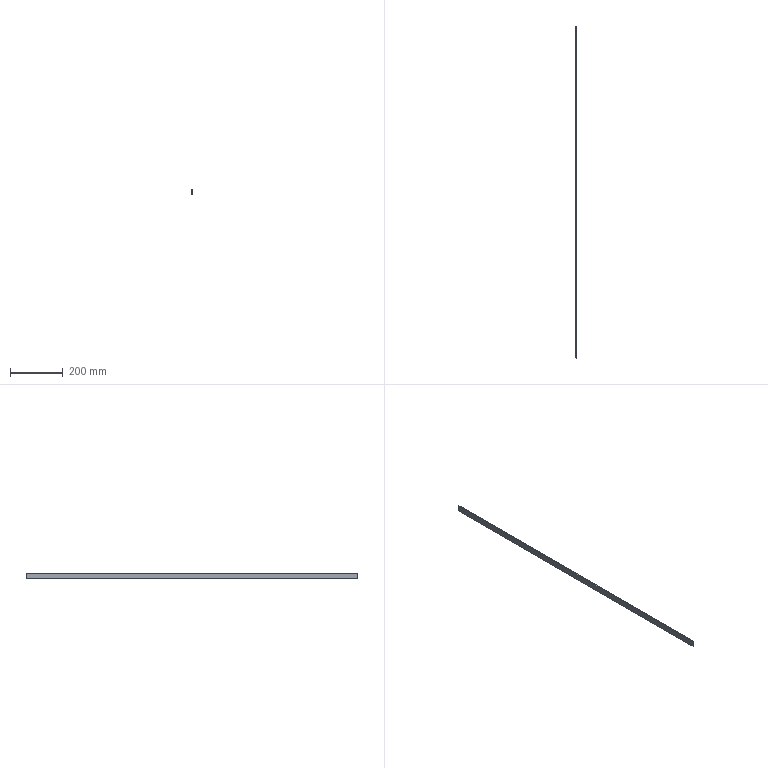Part | NX | features BREP 1 | 1 solid | 6 faces | box 4 x 1258 x 22 mm | volume 110734 mm3 | plane 6
STEP:
#1=CARTESIAN_POINT('',(597.336,-629.17,1234.305));
#2=VERTEX_POINT('',#1);
#3=CARTESIAN_POINT('',(597.336,-629.17,1256.305));
#4=VERTEX_POINT('',#3);
#5=CARTESIAN_POINT('',(597.336,-629.17,1245.305));
#6=DIRECTION('',(-0.000000043,0.,1.));
#7=VECTOR('',#6,1000.);
#8=LINE('',#5,#7);
#9=EDGE_CURVE('',#2,#4,#8,.T.);
#10=ORIENTED_EDGE('',*,*,#9,.T.);
#11=CARTESIAN_POINT('',(593.336,-629.17,1256.305));
#12=VERTEX_POINT('',#11);
#13=CARTESIAN_POINT('',(595.336,-629.17,1256.305));
#14=DIRECTION('',(1.,0.,0.000000043));
#15=VECTOR('',#14,1000.);
#16=LINE('',#13,#15);
#17=EDGE_CURVE('',#12,#4,#16,.T.);
#18=ORIENTED_EDGE('',*,*,#17,.F.);
#19=CARTESIAN_POINT('',(593.336,-629.17,1234.305));
#20=VERTEX_POINT('',#19);
#21=CARTESIAN_POINT('',(593.336,-629.17,1245.305));
#22=DIRECTION('',(0.000000043,0.,-1.));
#23=VECTOR('',#22,1000.);
#24=LINE('',#21,#23);
#25=EDGE_CURVE('',#12,#20,#24,.T.);
#26=ORIENTED_EDGE('',*,*,#25,.T.);
#27=CARTESIAN_POINT('',(595.336,-629.17,1234.305));
#28=DIRECTION('',(1.,0.,0.000000043));
#29=VECTOR('',#28,1000.);
#30=LINE('',#27,#29);
#31=EDGE_CURVE('',#20,#2,#30,.T.);
#32=ORIENTED_EDGE('',*,*,#31,.T.);
#33=EDGE_LOOP('',(#10,#18,#26,#32));
#34=FACE_BOUND('',#33,.T.);
#35=CARTESIAN_POINT('',(595.336,-629.17,401.145));
#36=DIRECTION('',(0.,-1.,0.));
#37=DIRECTION('',(1.,0.,0.000000043));
#38=AXIS2_PLACEMENT_3D('',#35,#36,#37);
#39=PLANE('',#38);
#40=ADVANCED_FACE('',(#34),#39,.T.);
#41=ORIENTED_EDGE('',*,*,#9,.F.);
#42=CARTESIAN_POINT('',(597.336,629.17,1234.305));
#43=VERTEX_POINT('',#42);
#44=CARTESIAN_POINT('',(597.336,0.,1234.305));
#45=DIRECTION('',(0.,-1.,0.));
#46=VECTOR('',#45,1000.);
#47=LINE('',#44,#46);
#48=EDGE_CURVE('',#43,#2,#47,.T.);
#49=ORIENTED_EDGE('',*,*,#48,.F.);
#50=CARTESIAN_POINT('',(597.336,629.17,1256.305));
#51=VERTEX_POINT('',#50);
#52=CARTESIAN_POINT('',(597.336,629.17,1245.305));
#53=DIRECTION('',(-0.000000043,0.,1.));
#54=VECTOR('',#53,1000.);
#55=LINE('',#52,#54);
#56=EDGE_CURVE('',#43,#51,#55,.T.);
#57=ORIENTED_EDGE('',*,*,#56,.T.);
#58=CARTESIAN_POINT('',(597.336,0.,1256.305));
#59=DIRECTION('',(0.,-1.,0.));
#60=VECTOR('',#59,1000.);
#61=LINE('',#58,#60);
#62=EDGE_CURVE('',#51,#4,#61,.T.);
#63=ORIENTED_EDGE('',*,*,#62,.T.);
#64=EDGE_LOOP('',(#41,#49,#57,#63));
#65=FACE_BOUND('',#64,.T.);
#66=CARTESIAN_POINT('',(597.336,629.17,1243.805));
#67=DIRECTION('',(1.,0.,0.000000043));
#68=DIRECTION('',(0.000000043,0.000003687,-1.));
#69=AXIS2_PLACEMENT_3D('',#66,#67,#68);
#70=PLANE('',#69);
#71=ADVANCED_FACE('',(#65),#70,.T.);
#72=ORIENTED_EDGE('',*,*,#62,.F.);
#73=CARTESIAN_POINT('',(593.336,629.17,1256.305));
#74=VERTEX_POINT('',#73);
#75=CARTESIAN_POINT('',(595.336,629.17,1256.305));
#76=DIRECTION('',(1.,0.,0.000000042));
#77=VECTOR('',#76,1000.);
#78=LINE('',#75,#77);
#79=EDGE_CURVE('',#74,#51,#78,.T.);
#80=ORIENTED_EDGE('',*,*,#79,.F.);
#81=CARTESIAN_POINT('',(593.336,0.,1256.305));
#82=DIRECTION('',(0.,-1.,0.));
#83=VECTOR('',#82,1000.);
#84=LINE('',#81,#83);
#85=EDGE_CURVE('',#74,#12,#84,.T.);
#86=ORIENTED_EDGE('',*,*,#85,.T.);
#87=ORIENTED_EDGE('',*,*,#17,.T.);
#88=EDGE_LOOP('',(#72,#80,#86,#87));
#89=FACE_BOUND('',#88,.T.);
#90=CARTESIAN_POINT('',(595.336,629.17,1256.305));
#91=DIRECTION('',(0.000000043,0.,-1.));
#92=DIRECTION('',(1.,0.,0.000000043));
#93=AXIS2_PLACEMENT_3D('',#90,#91,#92);
#94=PLANE('',#93);
#95=ADVANCED_FACE('',(#89),#94,.F.);
#96=ORIENTED_EDGE('',*,*,#85,.F.);
#97=CARTESIAN_POINT('',(593.336,629.17,1234.305));
#98=VERTEX_POINT('',#97);
#99=CARTESIAN_POINT('',(593.336,629.17,1245.305));
#100=DIRECTION('',(-0.000000043,0.,1.));
#101=VECTOR('',#100,1000.);
#102=LINE('',#99,#101);
#103=EDGE_CURVE('',#98,#74,#102,.T.);
#104=ORIENTED_EDGE('',*,*,#103,.F.);
#105=CARTESIAN_POINT('',(593.336,0.,1234.305));
#106=DIRECTION('',(0.,-1.,0.));
#107=VECTOR('',#106,1000.);
#108=LINE('',#105,#107);
#109=EDGE_CURVE('',#98,#20,#108,.T.);
#110=ORIENTED_EDGE('',*,*,#109,.T.);
#111=ORIENTED_EDGE('',*,*,#25,.F.);
#112=EDGE_LOOP('',(#96,#104,#110,#111));
#113=FACE_BOUND('',#112,.T.);
#114=CARTESIAN_POINT('',(593.336,629.17,1243.805));
#115=DIRECTION('',(1.,0.,0.000000043));
#116=DIRECTION('',(0.000000043,0.000003687,-1.));
#117=AXIS2_PLACEMENT_3D('',#114,#115,#116);
#118=PLANE('',#117);
#119=ADVANCED_FACE('',(#113),#118,.F.);
#120=ORIENTED_EDGE('',*,*,#31,.F.);
#121=ORIENTED_EDGE('',*,*,#109,.F.);
#122=CARTESIAN_POINT('',(595.336,629.17,1234.305));
#123=DIRECTION('',(1.,0.,0.000000042));
#124=VECTOR('',#123,1000.);
#125=LINE('',#122,#124);
#126=EDGE_CURVE('',#98,#43,#125,.T.);
#127=ORIENTED_EDGE('',*,*,#126,.T.);
#128=ORIENTED_EDGE('',*,*,#48,.T.);
#129=EDGE_LOOP('',(#120,#121,#127,#128));
#130=FACE_BOUND('',#129,.T.);
#131=CARTESIAN_POINT('',(595.336,629.17,1234.305));
#132=DIRECTION('',(0.000000043,0.,-1.));
#133=DIRECTION('',(1.,0.,0.000000043));
#134=AXIS2_PLACEMENT_3D('',#131,#132,#133);
#135=PLANE('',#134);
#136=ADVANCED_FACE('',(#130),#135,.T.);
#137=ORIENTED_EDGE('',*,*,#126,.F.);
#138=ORIENTED_EDGE('',*,*,#103,.T.);
#139=ORIENTED_EDGE('',*,*,#79,.T.);
#140=ORIENTED_EDGE('',*,*,#56,.F.);
#141=EDGE_LOOP('',(#137,#138,#139,#140));
#142=FACE_BOUND('',#141,.T.);
#143=CARTESIAN_POINT('',(595.336,629.17,401.145));
#144=DIRECTION('',(0.,-1.,0.));
#145=DIRECTION('',(1.,0.,0.000000043));
#146=AXIS2_PLACEMENT_3D('',#143,#144,#145);
#147=PLANE('',#146);
#148=ADVANCED_FACE('',(#142),#147,.F.);
#149=CLOSED_SHELL('',(#40,#71,#95,#119,#136,#148));
#150=MANIFOLD_SOLID_BREP('',#149);
#151=(LENGTH_UNIT()NAMED_UNIT(*)SI_UNIT(.MILLI.,.METRE.));
#152=UNCERTAINTY_MEASURE_WITH_UNIT(LENGTH_MEASURE(0.00001),#151,'','');
#153=(NAMED_UNIT(*)PLANE_ANGLE_UNIT()SI_UNIT($,.RADIAN.));
#154=(NAMED_UNIT(*)SI_UNIT($,.STERADIAN.)SOLID_ANGLE_UNIT());
#155=(GEOMETRIC_REPRESENTATION_CONTEXT(3)GLOBAL_UNCERTAINTY_ASSIGNED_CONTEXT((#152))GLOBAL_UNIT_ASSIGNED_CONTEXT((#151,#153,#154))REPRESENTATION_CONTEXT('',''));
#156=ADVANCED_BREP_SHAPE_REPRESENTATION('',(#150),#155);